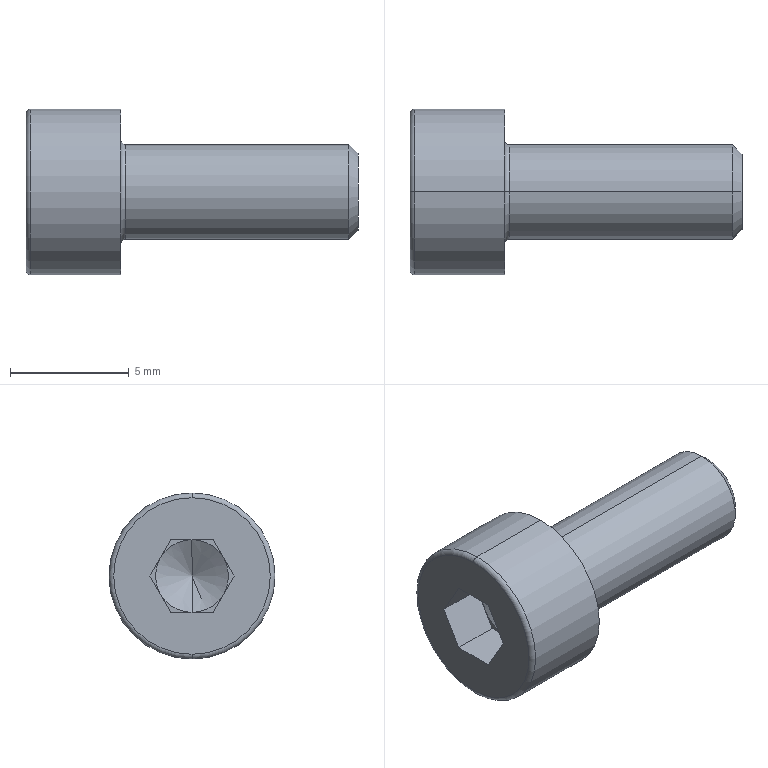Part | SolidWorks | features Fillet 2, RevCut 2, Attribute 1, Cut 1, LPattern 1, Revolution 1 | 1 solid | 27 faces | box 14 x 7 x 7 mm | volume 260.108 mm3 | plane 15 | cone 4 | torus 4 | cylinder 4 | commonest cylinder face diameters 4 x2 7 x2
STEP:
#1=CARTESIAN_POINT('',(2.887,0.,0.));
#2=VERTEX_POINT('',#1);
#3=CARTESIAN_POINT('',(2.,0.,1.535));
#4=VERTEX_POINT('',#3);
#5=CARTESIAN_POINT('',(2.,0.,1.536));
#6=DIRECTION('',(-0.5,0.,0.866));
#7=VECTOR('',#6,1000.);
#8=LINE('',#5,#7);
#9=EDGE_CURVE('',#2,#4,#8,.T.);
#10=ORIENTED_EDGE('',*,*,#9,.F.);
#11=CARTESIAN_POINT('',(2.,0.,-1.536));
#12=VERTEX_POINT('',#11);
#13=CARTESIAN_POINT('',(2.,0.,-1.536));
#14=DIRECTION('',(-0.5,0.,-0.866));
#15=VECTOR('',#14,1000.);
#16=LINE('',#13,#15);
#17=EDGE_CURVE('',#2,#12,#16,.T.);
#18=ORIENTED_EDGE('',*,*,#17,.T.);
#19=CARTESIAN_POINT('',(2.,-1.33,-0.7678));
#20=VERTEX_POINT('',#19);
#21=CARTESIAN_POINT('',(2.,0.,0.));
#22=DIRECTION('',(-1.,0.,0.));
#23=DIRECTION('',(0.,0.,1.));
#24=AXIS2_PLACEMENT_3D('',#21,#22,#23);
#25=CIRCLE('',#24,1.536);
#26=EDGE_CURVE('',#12,#20,#25,.T.);
#27=ORIENTED_EDGE('',*,*,#26,.T.);
#28=CARTESIAN_POINT('',(2.,-1.33,0.7678));
#29=VERTEX_POINT('',#28);
#30=CARTESIAN_POINT('',(2.,0.,0.));
#31=DIRECTION('',(-1.,0.,0.));
#32=DIRECTION('',(0.,0.,1.));
#33=AXIS2_PLACEMENT_3D('',#30,#31,#32);
#34=CIRCLE('',#33,1.536);
#35=EDGE_CURVE('',#20,#29,#34,.T.);
#36=ORIENTED_EDGE('',*,*,#35,.T.);
#37=CARTESIAN_POINT('',(2.,0.,0.));
#38=DIRECTION('',(-1.,0.,0.));
#39=DIRECTION('',(0.,0.,1.));
#40=AXIS2_PLACEMENT_3D('',#37,#38,#39);
#41=CIRCLE('',#40,1.536);
#42=EDGE_CURVE('',#29,#4,#41,.T.);
#43=ORIENTED_EDGE('',*,*,#42,.T.);
#44=EDGE_LOOP('',(#10,#18,#27,#36,#43));
#45=FACE_OUTER_BOUND('',#44,.T.);
#46=CARTESIAN_POINT('',(2.,0.,0.));
#47=DIRECTION('',(-1.,0.,0.));
#48=DIRECTION('',(0.,0.,1.));
#49=AXIS2_PLACEMENT_3D('',#46,#47,#48);
#50=CONICAL_SURFACE('',#49,1.536,1.047);
#51=ADVANCED_FACE('',(#45),#50,.F.);
#52=CARTESIAN_POINT('',(0.2,0.,-3.5));
#53=VERTEX_POINT('',#52);
#54=CARTESIAN_POINT('',(0.2,0.,3.5));
#55=VERTEX_POINT('',#54);
#56=CARTESIAN_POINT('',(0.2,0.,0.));
#57=DIRECTION('',(1.,0.,0.));
#58=DIRECTION('',(0.,0.,1.));
#59=AXIS2_PLACEMENT_3D('',#56,#57,#58);
#60=CIRCLE('',#59,3.5);
#61=EDGE_CURVE('',#53,#55,#60,.T.);
#62=ORIENTED_EDGE('',*,*,#61,.F.);
#63=CARTESIAN_POINT('',(0.,0.,-3.3));
#64=VERTEX_POINT('',#63);
#65=CARTESIAN_POINT('',(0.2,0.,-3.3));
#66=DIRECTION('',(0.,1.,0.));
#67=DIRECTION('',(0.,0.,1.));
#68=AXIS2_PLACEMENT_3D('',#65,#66,#67);
#69=CIRCLE('',#68,0.2);
#70=EDGE_CURVE('',#53,#64,#69,.T.);
#71=ORIENTED_EDGE('',*,*,#70,.T.);
#72=CARTESIAN_POINT('',(0.,0.,3.3));
#73=VERTEX_POINT('',#72);
#74=CARTESIAN_POINT('',(0.,0.,0.));
#75=DIRECTION('',(-1.,0.,0.));
#76=DIRECTION('',(0.,0.,1.));
#77=AXIS2_PLACEMENT_3D('',#74,#75,#76);
#78=CIRCLE('',#77,3.3);
#79=EDGE_CURVE('',#73,#64,#78,.T.);
#80=ORIENTED_EDGE('',*,*,#79,.F.);
#81=CARTESIAN_POINT('',(0.2,0.,3.3));
#82=DIRECTION('',(0.,-1.,0.));
#83=DIRECTION('',(0.,0.,-1.));
#84=AXIS2_PLACEMENT_3D('',#81,#82,#83);
#85=CIRCLE('',#84,0.2);
#86=EDGE_CURVE('',#55,#73,#85,.T.);
#87=ORIENTED_EDGE('',*,*,#86,.F.);
#88=EDGE_LOOP('',(#62,#71,#80,#87));
#89=FACE_OUTER_BOUND('',#88,.T.);
#90=CARTESIAN_POINT('',(0.2,0.,0.));
#91=DIRECTION('',(-1.,0.,0.));
#92=DIRECTION('',(0.,0.,1.));
#93=AXIS2_PLACEMENT_3D('',#90,#91,#92);
#94=TOROIDAL_SURFACE('',#93,3.3,0.2);
#95=ADVANCED_FACE('',(#89),#94,.T.);
#96=CARTESIAN_POINT('',(4.2,0.,2.));
#97=VERTEX_POINT('',#96);
#98=CARTESIAN_POINT('',(4.2,0.,-2.));
#99=VERTEX_POINT('',#98);
#100=CARTESIAN_POINT('',(4.2,0.,0.));
#101=DIRECTION('',(1.,0.,0.));
#102=DIRECTION('',(0.,0.,-1.));
#103=AXIS2_PLACEMENT_3D('',#100,#101,#102);
#104=CIRCLE('',#103,2.);
#105=EDGE_CURVE('',#97,#99,#104,.T.);
#106=ORIENTED_EDGE('',*,*,#105,.F.);
#107=CARTESIAN_POINT('',(4.,0.,2.2));
#108=VERTEX_POINT('',#107);
#109=CARTESIAN_POINT('',(4.2,0.,2.2));
#110=DIRECTION('',(0.,1.,0.));
#111=DIRECTION('',(0.,0.,1.));
#112=AXIS2_PLACEMENT_3D('',#109,#110,#111);
#113=CIRCLE('',#112,0.2);
#114=EDGE_CURVE('',#97,#108,#113,.T.);
#115=ORIENTED_EDGE('',*,*,#114,.T.);
#116=CARTESIAN_POINT('',(4.,0.,-2.2));
#117=VERTEX_POINT('',#116);
#118=CARTESIAN_POINT('',(4.,0.,0.));
#119=DIRECTION('',(-1.,0.,0.));
#120=DIRECTION('',(0.,0.,-1.));
#121=AXIS2_PLACEMENT_3D('',#118,#119,#120);
#122=CIRCLE('',#121,2.2);
#123=EDGE_CURVE('',#117,#108,#122,.T.);
#124=ORIENTED_EDGE('',*,*,#123,.F.);
#125=CARTESIAN_POINT('',(4.2,0.,-2.2));
#126=DIRECTION('',(0.,-1.,0.));
#127=DIRECTION('',(0.,0.,-1.));
#128=AXIS2_PLACEMENT_3D('',#125,#126,#127);
#129=CIRCLE('',#128,0.2);
#130=EDGE_CURVE('',#99,#117,#129,.T.);
#131=ORIENTED_EDGE('',*,*,#130,.F.);
#132=EDGE_LOOP('',(#106,#115,#124,#131));
#133=FACE_OUTER_BOUND('',#132,.T.);
#134=CARTESIAN_POINT('',(4.2,0.,0.));
#135=DIRECTION('',(1.,0.,0.));
#136=DIRECTION('',(0.,0.,-1.));
#137=AXIS2_PLACEMENT_3D('',#134,#135,#136);
#138=TOROIDAL_SURFACE('',#137,2.2,0.2);
#139=ADVANCED_FACE('',(#133),#138,.F.);
#140=CARTESIAN_POINT('',(14.,0.,1.61));
#141=VERTEX_POINT('',#140);
#142=CARTESIAN_POINT('',(14.,0.,-1.61));
#143=VERTEX_POINT('',#142);
#144=CARTESIAN_POINT('',(14.,0.,0.));
#145=DIRECTION('',(-1.,0.,0.));
#146=DIRECTION('',(0.,0.,1.));
#147=AXIS2_PLACEMENT_3D('',#144,#145,#146);
#148=CIRCLE('',#147,1.61);
#149=EDGE_CURVE('',#141,#143,#148,.T.);
#150=ORIENTED_EDGE('',*,*,#149,.T.);
#151=CARTESIAN_POINT('',(13.61,0.,-2.));
#152=VERTEX_POINT('',#151);
#153=CARTESIAN_POINT('',(14.,0.,-1.61));
#154=DIRECTION('',(-0.7071,0.,-0.7071));
#155=VECTOR('',#154,1000.);
#156=LINE('',#153,#155);
#157=EDGE_CURVE('',#143,#152,#156,.T.);
#158=ORIENTED_EDGE('',*,*,#157,.T.);
#159=CARTESIAN_POINT('',(13.61,0.,2.));
#160=VERTEX_POINT('',#159);
#161=CARTESIAN_POINT('',(13.61,0.,0.));
#162=DIRECTION('',(-1.,0.,0.));
#163=DIRECTION('',(0.,0.,1.));
#164=AXIS2_PLACEMENT_3D('',#161,#162,#163);
#165=CIRCLE('',#164,2.);
#166=EDGE_CURVE('',#160,#152,#165,.T.);
#167=ORIENTED_EDGE('',*,*,#166,.F.);
#168=CARTESIAN_POINT('',(14.,0.,1.61));
#169=DIRECTION('',(-0.7071,0.,0.7071));
#170=VECTOR('',#169,1000.);
#171=LINE('',#168,#170);
#172=EDGE_CURVE('',#141,#160,#171,.T.);
#173=ORIENTED_EDGE('',*,*,#172,.F.);
#174=EDGE_LOOP('',(#150,#158,#167,#173));
#175=FACE_OUTER_BOUND('',#174,.T.);
#176=CARTESIAN_POINT('',(14.,0.,0.));
#177=DIRECTION('',(-1.,0.,0.));
#178=DIRECTION('',(0.,0.,1.));
#179=AXIS2_PLACEMENT_3D('',#176,#177,#178);
#180=CONICAL_SURFACE('',#179,1.61,0.7854);
#181=ADVANCED_FACE('',(#175),#180,.T.);
#182=ORIENTED_EDGE('',*,*,#166,.T.);
#183=CARTESIAN_POINT('',(-31.75,0.,-2.));
#184=DIRECTION('',(-1.,0.,0.));
#185=VECTOR('',#184,1000.);
#186=LINE('',#183,#185);
#187=EDGE_CURVE('',#152,#99,#186,.T.);
#188=ORIENTED_EDGE('',*,*,#187,.T.);
#189=CARTESIAN_POINT('',(4.2,0.,0.));
#190=DIRECTION('',(1.,0.,0.));
#191=DIRECTION('',(0.,0.,-1.));
#192=AXIS2_PLACEMENT_3D('',#189,#190,#191);
#193=CIRCLE('',#192,2.);
#194=EDGE_CURVE('',#99,#97,#193,.T.);
#195=ORIENTED_EDGE('',*,*,#194,.T.);
#196=CARTESIAN_POINT('',(-31.75,0.,2.));
#197=DIRECTION('',(-1.,0.,0.));
#198=VECTOR('',#197,1000.);
#199=LINE('',#196,#198);
#200=EDGE_CURVE('',#160,#97,#199,.T.);
#201=ORIENTED_EDGE('',*,*,#200,.F.);
#202=EDGE_LOOP('',(#182,#188,#195,#201));
#203=FACE_OUTER_BOUND('',#202,.T.);
#204=CARTESIAN_POINT('',(-31.75,0.,0.));
#205=DIRECTION('',(-1.,0.,0.));
#206=DIRECTION('',(0.,0.,1.));
#207=AXIS2_PLACEMENT_3D('',#204,#205,#206);
#208=CYLINDRICAL_SURFACE('',#207,2.);
#209=ADVANCED_FACE('',(#203),#208,.T.);
#210=CARTESIAN_POINT('',(4.,0.,3.5));
#211=VERTEX_POINT('',#210);
#212=CARTESIAN_POINT('',(4.,0.,-3.5));
#213=VERTEX_POINT('',#212);
#214=CARTESIAN_POINT('',(4.,0.,0.));
#215=DIRECTION('',(-1.,0.,0.));
#216=DIRECTION('',(0.,0.,1.));
#217=AXIS2_PLACEMENT_3D('',#214,#215,#216);
#218=CIRCLE('',#217,3.5);
#219=EDGE_CURVE('',#211,#213,#218,.T.);
#220=ORIENTED_EDGE('',*,*,#219,.T.);
#221=CARTESIAN_POINT('',(-31.75,0.,-3.5));
#222=DIRECTION('',(-1.,0.,0.));
#223=VECTOR('',#222,1000.);
#224=LINE('',#221,#223);
#225=EDGE_CURVE('',#213,#53,#224,.T.);
#226=ORIENTED_EDGE('',*,*,#225,.T.);
#227=ORIENTED_EDGE('',*,*,#61,.T.);
#228=CARTESIAN_POINT('',(-31.75,0.,3.5));
#229=DIRECTION('',(-1.,0.,0.));
#230=VECTOR('',#229,1000.);
#231=LINE('',#228,#230);
#232=EDGE_CURVE('',#211,#55,#231,.T.);
#233=ORIENTED_EDGE('',*,*,#232,.F.);
#234=EDGE_LOOP('',(#220,#226,#227,#233));
#235=FACE_OUTER_BOUND('',#234,.T.);
#236=CARTESIAN_POINT('',(-31.75,0.,0.));
#237=DIRECTION('',(-1.,0.,0.));
#238=DIRECTION('',(0.,0.,1.));
#239=AXIS2_PLACEMENT_3D('',#236,#237,#238);
#240=CYLINDRICAL_SURFACE('',#239,3.5);
#241=ADVANCED_FACE('',(#235),#240,.T.);
#242=CARTESIAN_POINT('',(0.,1.773,0.));
#243=VERTEX_POINT('',#242);
#244=CARTESIAN_POINT('',(0.,0.8865,1.535));
#245=VERTEX_POINT('',#244);
#246=CARTESIAN_POINT('',(0.,1.773,0.));
#247=DIRECTION('',(0.,-0.5,0.866));
#248=VECTOR('',#247,1000.);
#249=LINE('',#246,#248);
#250=EDGE_CURVE('',#243,#245,#249,.T.);
#251=ORIENTED_EDGE('',*,*,#250,.T.);
#252=CARTESIAN_POINT('',(0.,-0.8865,1.535));
#253=VERTEX_POINT('',#252);
#254=CARTESIAN_POINT('',(0.,-0.8865,1.535));
#255=DIRECTION('',(0.,1.,0.));
#256=VECTOR('',#255,1000.);
#257=LINE('',#254,#256);
#258=EDGE_CURVE('',#253,#245,#257,.T.);
#259=ORIENTED_EDGE('',*,*,#258,.F.);
#260=CARTESIAN_POINT('',(0.,-1.773,0.));
#261=VERTEX_POINT('',#260);
#262=CARTESIAN_POINT('',(0.,-0.8865,1.535));
#263=DIRECTION('',(0.,-0.5,-0.866));
#264=VECTOR('',#263,1000.);
#265=LINE('',#262,#264);
#266=EDGE_CURVE('',#253,#261,#265,.T.);
#267=ORIENTED_EDGE('',*,*,#266,.T.);
#268=CARTESIAN_POINT('',(0.,-0.8865,-1.536));
#269=VERTEX_POINT('',#268);
#270=CARTESIAN_POINT('',(0.,-1.773,0.));
#271=DIRECTION('',(0.,0.5,-0.866));
#272=VECTOR('',#271,1000.);
#273=LINE('',#270,#272);
#274=EDGE_CURVE('',#261,#269,#273,.T.);
#275=ORIENTED_EDGE('',*,*,#274,.T.);
#276=CARTESIAN_POINT('',(0.,0.8865,-1.536));
#277=VERTEX_POINT('',#276);
#278=CARTESIAN_POINT('',(0.,0.8865,-1.536));
#279=DIRECTION('',(0.,-1.,0.));
#280=VECTOR('',#279,1000.);
#281=LINE('',#278,#280);
#282=EDGE_CURVE('',#277,#269,#281,.T.);
#283=ORIENTED_EDGE('',*,*,#282,.F.);
#284=CARTESIAN_POINT('',(0.,1.773,0.));
#285=DIRECTION('',(0.,-0.5,-0.866));
#286=VECTOR('',#285,1000.);
#287=LINE('',#284,#286);
#288=EDGE_CURVE('',#243,#277,#287,.T.);
#289=ORIENTED_EDGE('',*,*,#288,.F.);
#290=EDGE_LOOP('',(#251,#259,#267,#275,#283,#289));
#291=FACE_BOUND('',#290,.T.);
#292=ORIENTED_EDGE('',*,*,#79,.T.);
#293=CARTESIAN_POINT('',(0.,0.,0.));
#294=DIRECTION('',(-1.,0.,0.));
#295=DIRECTION('',(0.,0.,1.));
#296=AXIS2_PLACEMENT_3D('',#293,#294,#295);
#297=CIRCLE('',#296,3.3);
#298=EDGE_CURVE('',#64,#73,#297,.T.);
#299=ORIENTED_EDGE('',*,*,#298,.T.);
#300=EDGE_LOOP('',(#292,#299));
#301=FACE_OUTER_BOUND('',#300,.T.);
#302=CARTESIAN_POINT('',(0.,0.,0.));
#303=DIRECTION('',(-1.,0.,0.));
#304=DIRECTION('',(0.,0.,1.));
#305=AXIS2_PLACEMENT_3D('',#302,#303,#304);
#306=PLANE('',#305);
#307=ADVANCED_FACE('',(#291,#301),#306,.T.);
#308=ORIENTED_EDGE('',*,*,#225,.F.);
#309=CARTESIAN_POINT('',(4.,0.,0.));
#310=DIRECTION('',(-1.,0.,0.));
#311=DIRECTION('',(0.,0.,1.));
#312=AXIS2_PLACEMENT_3D('',#309,#310,#311);
#313=CIRCLE('',#312,3.5);
#314=EDGE_CURVE('',#213,#211,#313,.T.);
#315=ORIENTED_EDGE('',*,*,#314,.T.);
#316=ORIENTED_EDGE('',*,*,#232,.T.);
#317=CARTESIAN_POINT('',(0.2,0.,0.));
#318=DIRECTION('',(1.,0.,0.));
#319=DIRECTION('',(0.,0.,1.));
#320=AXIS2_PLACEMENT_3D('',#317,#318,#319);
#321=CIRCLE('',#320,3.5);
#322=EDGE_CURVE('',#55,#53,#321,.T.);
#323=ORIENTED_EDGE('',*,*,#322,.T.);
#324=EDGE_LOOP('',(#308,#315,#316,#323));
#325=FACE_OUTER_BOUND('',#324,.T.);
#326=CARTESIAN_POINT('',(-31.75,0.,0.));
#327=DIRECTION('',(-1.,0.,0.));
#328=DIRECTION('',(0.,0.,1.));
#329=AXIS2_PLACEMENT_3D('',#326,#327,#328);
#330=CYLINDRICAL_SURFACE('',#329,3.5);
#331=ADVANCED_FACE('',(#325),#330,.T.);
#332=ORIENTED_EDGE('',*,*,#123,.T.);
#333=CARTESIAN_POINT('',(4.,0.,0.));
#334=DIRECTION('',(-1.,0.,0.));
#335=DIRECTION('',(0.,0.,-1.));
#336=AXIS2_PLACEMENT_3D('',#333,#334,#335);
#337=CIRCLE('',#336,2.2);
#338=EDGE_CURVE('',#108,#117,#337,.T.);
#339=ORIENTED_EDGE('',*,*,#338,.T.);
#340=EDGE_LOOP('',(#332,#339));
#341=FACE_BOUND('',#340,.T.);
#342=ORIENTED_EDGE('',*,*,#219,.F.);
#343=ORIENTED_EDGE('',*,*,#314,.F.);
#344=EDGE_LOOP('',(#342,#343));
#345=FACE_OUTER_BOUND('',#344,.T.);
#346=CARTESIAN_POINT('',(4.,3.5,0.));
#347=DIRECTION('',(1.,0.,0.));
#348=DIRECTION('',(0.,0.,-1.));
#349=AXIS2_PLACEMENT_3D('',#346,#347,#348);
#350=PLANE('',#349);
#351=ADVANCED_FACE('',(#341,#345),#350,.T.);
#352=ORIENTED_EDGE('',*,*,#187,.F.);
#353=CARTESIAN_POINT('',(13.61,0.,0.));
#354=DIRECTION('',(-1.,0.,0.));
#355=DIRECTION('',(0.,0.,1.));
#356=AXIS2_PLACEMENT_3D('',#353,#354,#355);
#357=CIRCLE('',#356,2.);
#358=EDGE_CURVE('',#152,#160,#357,.T.);
#359=ORIENTED_EDGE('',*,*,#358,.T.);
#360=ORIENTED_EDGE('',*,*,#200,.T.);
#361=ORIENTED_EDGE('',*,*,#105,.T.);
#362=EDGE_LOOP('',(#352,#359,#360,#361));
#363=FACE_OUTER_BOUND('',#362,.T.);
#364=CARTESIAN_POINT('',(-31.75,0.,0.));
#365=DIRECTION('',(-1.,0.,0.));
#366=DIRECTION('',(0.,0.,1.));
#367=AXIS2_PLACEMENT_3D('',#364,#365,#366);
#368=CYLINDRICAL_SURFACE('',#367,2.);
#369=ADVANCED_FACE('',(#363),#368,.T.);
#370=ORIENTED_EDGE('',*,*,#157,.F.);
#371=CARTESIAN_POINT('',(14.,0.,0.));
#372=DIRECTION('',(-1.,0.,0.));
#373=DIRECTION('',(0.,0.,1.));
#374=AXIS2_PLACEMENT_3D('',#371,#372,#373);
#375=CIRCLE('',#374,1.61);
#376=EDGE_CURVE('',#143,#141,#375,.T.);
#377=ORIENTED_EDGE('',*,*,#376,.T.);
#378=ORIENTED_EDGE('',*,*,#172,.T.);
#379=ORIENTED_EDGE('',*,*,#358,.F.);
#380=EDGE_LOOP('',(#370,#377,#378,#379));
#381=FACE_OUTER_BOUND('',#380,.T.);
#382=CARTESIAN_POINT('',(14.,0.,0.));
#383=DIRECTION('',(-1.,0.,0.));
#384=DIRECTION('',(0.,0.,1.));
#385=AXIS2_PLACEMENT_3D('',#382,#383,#384);
#386=CONICAL_SURFACE('',#385,1.61,0.7854);
#387=ADVANCED_FACE('',(#381),#386,.T.);
#388=ORIENTED_EDGE('',*,*,#149,.F.);
#389=ORIENTED_EDGE('',*,*,#376,.F.);
#390=EDGE_LOOP('',(#388,#389));
#391=FACE_OUTER_BOUND('',#390,.T.);
#392=CARTESIAN_POINT('',(14.,1.61,0.));
#393=DIRECTION('',(1.,0.,0.));
#394=DIRECTION('',(0.,0.,-1.));
#395=AXIS2_PLACEMENT_3D('',#392,#393,#394);
#396=PLANE('',#395);
#397=ADVANCED_FACE('',(#391),#396,.T.);
#398=ORIENTED_EDGE('',*,*,#114,.F.);
#399=ORIENTED_EDGE('',*,*,#194,.F.);
#400=ORIENTED_EDGE('',*,*,#130,.T.);
#401=ORIENTED_EDGE('',*,*,#338,.F.);
#402=EDGE_LOOP('',(#398,#399,#400,#401));
#403=FACE_OUTER_BOUND('',#402,.T.);
#404=CARTESIAN_POINT('',(4.2,0.,0.));
#405=DIRECTION('',(1.,0.,0.));
#406=DIRECTION('',(0.,0.,-1.));
#407=AXIS2_PLACEMENT_3D('',#404,#405,#406);
#408=TOROIDAL_SURFACE('',#407,2.2,0.2);
#409=ADVANCED_FACE('',(#403),#408,.F.);
#410=ORIENTED_EDGE('',*,*,#70,.F.);
#411=ORIENTED_EDGE('',*,*,#322,.F.);
#412=ORIENTED_EDGE('',*,*,#86,.T.);
#413=ORIENTED_EDGE('',*,*,#298,.F.);
#414=EDGE_LOOP('',(#410,#411,#412,#413));
#415=FACE_OUTER_BOUND('',#414,.T.);
#416=CARTESIAN_POINT('',(0.2,0.,0.));
#417=DIRECTION('',(-1.,0.,0.));
#418=DIRECTION('',(0.,0.,1.));
#419=AXIS2_PLACEMENT_3D('',#416,#417,#418);
#420=TOROIDAL_SURFACE('',#419,3.3,0.2);
#421=ADVANCED_FACE('',(#415),#420,.T.);
#422=ORIENTED_EDGE('',*,*,#250,.F.);
#423=CARTESIAN_POINT('',(2.,1.773,0.));
#424=VERTEX_POINT('',#423);
#425=CARTESIAN_POINT('',(2.,1.773,0.));
#426=DIRECTION('',(-1.,0.,0.));
#427=VECTOR('',#426,1000.);
#428=LINE('',#425,#427);
#429=EDGE_CURVE('',#424,#243,#428,.T.);
#430=ORIENTED_EDGE('',*,*,#429,.F.);
#431=CARTESIAN_POINT('',(2.,1.33,0.7677));
#432=VERTEX_POINT('',#431);
#433=CARTESIAN_POINT('',(2.,1.773,0.));
#434=DIRECTION('',(0.,-0.5,0.866));
#435=VECTOR('',#434,1000.);
#436=LINE('',#433,#435);
#437=EDGE_CURVE('',#424,#432,#436,.T.);
#438=ORIENTED_EDGE('',*,*,#437,.T.);
#439=CARTESIAN_POINT('',(2.,0.8865,1.535));
#440=VERTEX_POINT('',#439);
#441=CARTESIAN_POINT('',(2.,1.773,0.));
#442=DIRECTION('',(0.,-0.5,0.866));
#443=VECTOR('',#442,1000.);
#444=LINE('',#441,#443);
#445=EDGE_CURVE('',#432,#440,#444,.T.);
#446=ORIENTED_EDGE('',*,*,#445,.T.);
#447=CARTESIAN_POINT('',(2.,0.8865,1.535));
#448=DIRECTION('',(-1.,0.,0.));
#449=VECTOR('',#448,1000.);
#450=LINE('',#447,#449);
#451=EDGE_CURVE('',#440,#245,#450,.T.);
#452=ORIENTED_EDGE('',*,*,#451,.T.);
#453=EDGE_LOOP('',(#422,#430,#438,#446,#452));
#454=FACE_OUTER_BOUND('',#453,.T.);
#455=CARTESIAN_POINT('',(2.,1.773,0.));
#456=DIRECTION('',(0.,-0.866,-0.5));
#457=DIRECTION('',(0.,0.5,-0.866));
#458=AXIS2_PLACEMENT_3D('',#455,#456,#457);
#459=PLANE('',#458);
#460=ADVANCED_FACE('',(#454),#459,.T.);
#461=ORIENTED_EDGE('',*,*,#258,.T.);
#462=ORIENTED_EDGE('',*,*,#451,.F.);
#463=CARTESIAN_POINT('',(2.,-0.8865,1.535));
#464=DIRECTION('',(0.,1.,0.));
#465=VECTOR('',#464,1000.);
#466=LINE('',#463,#465);
#467=EDGE_CURVE('',#4,#440,#466,.T.);
#468=ORIENTED_EDGE('',*,*,#467,.F.);
#469=CARTESIAN_POINT('',(2.,-0.8865,1.535));
#470=VERTEX_POINT('',#469);
#471=CARTESIAN_POINT('',(2.,-0.8865,1.535));
#472=DIRECTION('',(0.,1.,0.));
#473=VECTOR('',#472,1000.);
#474=LINE('',#471,#473);
#475=EDGE_CURVE('',#470,#4,#474,.T.);
#476=ORIENTED_EDGE('',*,*,#475,.F.);
#477=CARTESIAN_POINT('',(2.,-0.8865,1.535));
#478=DIRECTION('',(-1.,0.,0.));
#479=VECTOR('',#478,1000.);
#480=LINE('',#477,#479);
#481=EDGE_CURVE('',#470,#253,#480,.T.);
#482=ORIENTED_EDGE('',*,*,#481,.T.);
#483=EDGE_LOOP('',(#461,#462,#468,#476,#482));
#484=FACE_OUTER_BOUND('',#483,.T.);
#485=CARTESIAN_POINT('',(2.,-0.8865,1.535));
#486=DIRECTION('',(0.,0.,1.));
#487=DIRECTION('',(0.,-1.,0.));
#488=AXIS2_PLACEMENT_3D('',#485,#486,#487);
#489=PLANE('',#488);
#490=ADVANCED_FACE('',(#484),#489,.F.);
#491=ORIENTED_EDGE('',*,*,#266,.F.);
#492=ORIENTED_EDGE('',*,*,#481,.F.);
#493=CARTESIAN_POINT('',(2.,-0.8865,1.535));
#494=DIRECTION('',(0.,-0.5,-0.866));
#495=VECTOR('',#494,1000.);
#496=LINE('',#493,#495);
#497=EDGE_CURVE('',#470,#29,#496,.T.);
#498=ORIENTED_EDGE('',*,*,#497,.T.);
#499=CARTESIAN_POINT('',(2.,-1.773,0.));
#500=VERTEX_POINT('',#499);
#501=CARTESIAN_POINT('',(2.,-0.8865,1.535));
#502=DIRECTION('',(0.,-0.5,-0.866));
#503=VECTOR('',#502,1000.);
#504=LINE('',#501,#503);
#505=EDGE_CURVE('',#29,#500,#504,.T.);
#506=ORIENTED_EDGE('',*,*,#505,.T.);
#507=CARTESIAN_POINT('',(2.,-1.773,0.));
#508=DIRECTION('',(-1.,0.,0.));
#509=VECTOR('',#508,1000.);
#510=LINE('',#507,#509);
#511=EDGE_CURVE('',#500,#261,#510,.T.);
#512=ORIENTED_EDGE('',*,*,#511,.T.);
#513=EDGE_LOOP('',(#491,#492,#498,#506,#512));
#514=FACE_OUTER_BOUND('',#513,.T.);
#515=CARTESIAN_POINT('',(2.,-0.8865,1.535));
#516=DIRECTION('',(0.,0.866,-0.5));
#517=DIRECTION('',(0.,0.5,0.866));
#518=AXIS2_PLACEMENT_3D('',#515,#516,#517);
#519=PLANE('',#518);
#520=ADVANCED_FACE('',(#514),#519,.T.);
#521=ORIENTED_EDGE('',*,*,#274,.F.);
#522=ORIENTED_EDGE('',*,*,#511,.F.);
#523=CARTESIAN_POINT('',(2.,-1.773,0.));
#524=DIRECTION('',(0.,0.5,-0.866));
#525=VECTOR('',#524,1000.);
#526=LINE('',#523,#525);
#527=EDGE_CURVE('',#500,#20,#526,.T.);
#528=ORIENTED_EDGE('',*,*,#527,.T.);
#529=CARTESIAN_POINT('',(2.,-0.8865,-1.536));
#530=VERTEX_POINT('',#529);
#531=CARTESIAN_POINT('',(2.,-1.773,0.));
#532=DIRECTION('',(0.,0.5,-0.866));
#533=VECTOR('',#532,1000.);
#534=LINE('',#531,#533);
#535=EDGE_CURVE('',#20,#530,#534,.T.);
#536=ORIENTED_EDGE('',*,*,#535,.T.);
#537=CARTESIAN_POINT('',(2.,-0.8865,-1.536));
#538=DIRECTION('',(-1.,0.,0.));
#539=VECTOR('',#538,1000.);
#540=LINE('',#537,#539);
#541=EDGE_CURVE('',#530,#269,#540,.T.);
#542=ORIENTED_EDGE('',*,*,#541,.T.);
#543=EDGE_LOOP('',(#521,#522,#528,#536,#542));
#544=FACE_OUTER_BOUND('',#543,.T.);
#545=CARTESIAN_POINT('',(2.,-1.773,0.));
#546=DIRECTION('',(0.,0.866,0.5));
#547=DIRECTION('',(0.,-0.5,0.866));
#548=AXIS2_PLACEMENT_3D('',#545,#546,#547);
#549=PLANE('',#548);
#550=ADVANCED_FACE('',(#544),#549,.T.);
#551=ORIENTED_EDGE('',*,*,#282,.T.);
#552=ORIENTED_EDGE('',*,*,#541,.F.);
#553=CARTESIAN_POINT('',(2.,0.8865,-1.536));
#554=DIRECTION('',(0.,-1.,0.));
#555=VECTOR('',#554,1000.);
#556=LINE('',#553,#555);
#557=EDGE_CURVE('',#12,#530,#556,.T.);
#558=ORIENTED_EDGE('',*,*,#557,.F.);
#559=CARTESIAN_POINT('',(2.,0.8865,-1.536));
#560=VERTEX_POINT('',#559);
#561=CARTESIAN_POINT('',(2.,0.8865,-1.536));
#562=DIRECTION('',(0.,-1.,0.));
#563=VECTOR('',#562,1000.);
#564=LINE('',#561,#563);
#565=EDGE_CURVE('',#560,#12,#564,.T.);
#566=ORIENTED_EDGE('',*,*,#565,.F.);
#567=CARTESIAN_POINT('',(2.,0.8865,-1.536));
#568=DIRECTION('',(-1.,0.,0.));
#569=VECTOR('',#568,1000.);
#570=LINE('',#567,#569);
#571=EDGE_CURVE('',#560,#277,#570,.T.);
#572=ORIENTED_EDGE('',*,*,#571,.T.);
#573=EDGE_LOOP('',(#551,#552,#558,#566,#572));
#574=FACE_OUTER_BOUND('',#573,.T.);
#575=CARTESIAN_POINT('',(2.,0.8865,-1.536));
#576=DIRECTION('',(0.,0.,-1.));
#577=DIRECTION('',(0.,1.,0.));
#578=AXIS2_PLACEMENT_3D('',#575,#576,#577);
#579=PLANE('',#578);
#580=ADVANCED_FACE('',(#574),#579,.F.);
#581=ORIENTED_EDGE('',*,*,#288,.T.);
#582=ORIENTED_EDGE('',*,*,#571,.F.);
#583=CARTESIAN_POINT('',(2.,1.33,-0.7678));
#584=VERTEX_POINT('',#583);
#585=CARTESIAN_POINT('',(2.,1.773,0.));
#586=DIRECTION('',(0.,-0.5,-0.866));
#587=VECTOR('',#586,1000.);
#588=LINE('',#585,#587);
#589=EDGE_CURVE('',#584,#560,#588,.T.);
#590=ORIENTED_EDGE('',*,*,#589,.F.);
#591=CARTESIAN_POINT('',(2.,1.773,0.));
#592=DIRECTION('',(0.,-0.5,-0.866));
#593=VECTOR('',#592,1000.);
#594=LINE('',#591,#593);
#595=EDGE_CURVE('',#424,#584,#594,.T.);
#596=ORIENTED_EDGE('',*,*,#595,.F.);
#597=ORIENTED_EDGE('',*,*,#429,.T.);
#598=EDGE_LOOP('',(#581,#582,#590,#596,#597));
#599=FACE_OUTER_BOUND('',#598,.T.);
#600=CARTESIAN_POINT('',(2.,1.773,0.));
#601=DIRECTION('',(0.,0.866,-0.5));
#602=DIRECTION('',(0.,0.5,0.866));
#603=AXIS2_PLACEMENT_3D('',#600,#601,#602);
#604=PLANE('',#603);
#605=ADVANCED_FACE('',(#599),#604,.F.);
#606=ORIENTED_EDGE('',*,*,#557,.T.);
#607=ORIENTED_EDGE('',*,*,#535,.F.);
#608=ORIENTED_EDGE('',*,*,#26,.F.);
#609=EDGE_LOOP('',(#606,#607,#608));
#610=FACE_OUTER_BOUND('',#609,.T.);
#611=CARTESIAN_POINT('',(2.,1.773,0.));
#612=DIRECTION('',(1.,0.,0.));
#613=DIRECTION('',(0.,0.,-1.));
#614=AXIS2_PLACEMENT_3D('',#611,#612,#613);
#615=PLANE('',#614);
#616=ADVANCED_FACE('',(#610),#615,.F.);
#617=ORIENTED_EDGE('',*,*,#527,.F.);
#618=ORIENTED_EDGE('',*,*,#505,.F.);
#619=ORIENTED_EDGE('',*,*,#35,.F.);
#620=EDGE_LOOP('',(#617,#618,#619));
#621=FACE_OUTER_BOUND('',#620,.T.);
#622=CARTESIAN_POINT('',(2.,1.773,0.));
#623=DIRECTION('',(1.,0.,0.));
#624=DIRECTION('',(0.,0.,-1.));
#625=AXIS2_PLACEMENT_3D('',#622,#623,#624);
#626=PLANE('',#625);
#627=ADVANCED_FACE('',(#621),#626,.F.);
#628=ORIENTED_EDGE('',*,*,#497,.F.);
#629=ORIENTED_EDGE('',*,*,#475,.T.);
#630=ORIENTED_EDGE('',*,*,#42,.F.);
#631=EDGE_LOOP('',(#628,#629,#630));
#632=FACE_OUTER_BOUND('',#631,.T.);
#633=CARTESIAN_POINT('',(2.,1.773,0.));
#634=DIRECTION('',(1.,0.,0.));
#635=DIRECTION('',(0.,0.,-1.));
#636=AXIS2_PLACEMENT_3D('',#633,#634,#635);
#637=PLANE('',#636);
#638=ADVANCED_FACE('',(#632),#637,.F.);
#639=ORIENTED_EDGE('',*,*,#467,.T.);
#640=ORIENTED_EDGE('',*,*,#445,.F.);
#641=CARTESIAN_POINT('',(2.,0.,0.));
#642=DIRECTION('',(-1.,0.,0.));
#643=DIRECTION('',(0.,0.,1.));
#644=AXIS2_PLACEMENT_3D('',#641,#642,#643);
#645=CIRCLE('',#644,1.536);
#646=EDGE_CURVE('',#4,#432,#645,.T.);
#647=ORIENTED_EDGE('',*,*,#646,.F.);
#648=EDGE_LOOP('',(#639,#640,#647));
#649=FACE_OUTER_BOUND('',#648,.T.);
#650=CARTESIAN_POINT('',(2.,1.773,0.));
#651=DIRECTION('',(1.,0.,0.));
#652=DIRECTION('',(0.,0.,-1.));
#653=AXIS2_PLACEMENT_3D('',#650,#651,#652);
#654=PLANE('',#653);
#655=ADVANCED_FACE('',(#649),#654,.F.);
#656=ORIENTED_EDGE('',*,*,#437,.F.);
#657=ORIENTED_EDGE('',*,*,#595,.T.);
#658=CARTESIAN_POINT('',(2.,0.,0.));
#659=DIRECTION('',(-1.,0.,0.));
#660=DIRECTION('',(0.,0.,1.));
#661=AXIS2_PLACEMENT_3D('',#658,#659,#660);
#662=CIRCLE('',#661,1.536);
#663=EDGE_CURVE('',#432,#584,#662,.T.);
#664=ORIENTED_EDGE('',*,*,#663,.F.);
#665=EDGE_LOOP('',(#656,#657,#664));
#666=FACE_OUTER_BOUND('',#665,.T.);
#667=CARTESIAN_POINT('',(2.,1.773,0.));
#668=DIRECTION('',(1.,0.,0.));
#669=DIRECTION('',(0.,0.,-1.));
#670=AXIS2_PLACEMENT_3D('',#667,#668,#669);
#671=PLANE('',#670);
#672=ADVANCED_FACE('',(#666),#671,.F.);
#673=ORIENTED_EDGE('',*,*,#589,.T.);
#674=ORIENTED_EDGE('',*,*,#565,.T.);
#675=CARTESIAN_POINT('',(2.,0.,0.));
#676=DIRECTION('',(-1.,0.,0.));
#677=DIRECTION('',(0.,0.,1.));
#678=AXIS2_PLACEMENT_3D('',#675,#676,#677);
#679=CIRCLE('',#678,1.536);
#680=EDGE_CURVE('',#584,#12,#679,.T.);
#681=ORIENTED_EDGE('',*,*,#680,.F.);
#682=EDGE_LOOP('',(#673,#674,#681));
#683=FACE_OUTER_BOUND('',#682,.T.);
#684=CARTESIAN_POINT('',(2.,1.773,0.));
#685=DIRECTION('',(1.,0.,0.));
#686=DIRECTION('',(0.,0.,-1.));
#687=AXIS2_PLACEMENT_3D('',#684,#685,#686);
#688=PLANE('',#687);
#689=ADVANCED_FACE('',(#683),#688,.F.);
#690=ORIENTED_EDGE('',*,*,#17,.F.);
#691=ORIENTED_EDGE('',*,*,#9,.T.);
#692=ORIENTED_EDGE('',*,*,#646,.T.);
#693=ORIENTED_EDGE('',*,*,#663,.T.);
#694=ORIENTED_EDGE('',*,*,#680,.T.);
#695=EDGE_LOOP('',(#690,#691,#692,#693,#694));
#696=FACE_OUTER_BOUND('',#695,.T.);
#697=CARTESIAN_POINT('',(2.,0.,0.));
#698=DIRECTION('',(-1.,0.,0.));
#699=DIRECTION('',(0.,0.,1.));
#700=AXIS2_PLACEMENT_3D('',#697,#698,#699);
#701=CONICAL_SURFACE('',#700,1.536,1.047);
#702=ADVANCED_FACE('',(#696),#701,.F.);
#703=CLOSED_SHELL('',(#51,#95,#139,#181,#209,#241,#307,#331,#351,#369,#387,#397,#409,#421,#460,#490,#520,#550,#580,#605,#616,#627,#638,#655,#672,#689,#702));
#704=MANIFOLD_SOLID_BREP('',#703);
#705=CARTESIAN_POINT('',(0.,0.,0.));
#706=DIRECTION('',(0.,0.,1.));
#707=DIRECTION('',(1.,0.,0.));
#708=AXIS2_PLACEMENT_3D('',#705,#706,#707);
#709=(LENGTH_UNIT()NAMED_UNIT(*)SI_UNIT(.MILLI.,.METRE.));
#710=UNCERTAINTY_MEASURE_WITH_UNIT(LENGTH_MEASURE(0.00001),#709,'','');
#711=(NAMED_UNIT(*)PLANE_ANGLE_UNIT()SI_UNIT($,.RADIAN.));
#712=(NAMED_UNIT(*)SI_UNIT($,.STERADIAN.)SOLID_ANGLE_UNIT());
#713=(GEOMETRIC_REPRESENTATION_CONTEXT(3)GLOBAL_UNCERTAINTY_ASSIGNED_CONTEXT((#710))GLOBAL_UNIT_ASSIGNED_CONTEXT((#709,#711,#712))REPRESENTATION_CONTEXT('',''));
#714=ADVANCED_BREP_SHAPE_REPRESENTATION('',(#704,#708),#713);